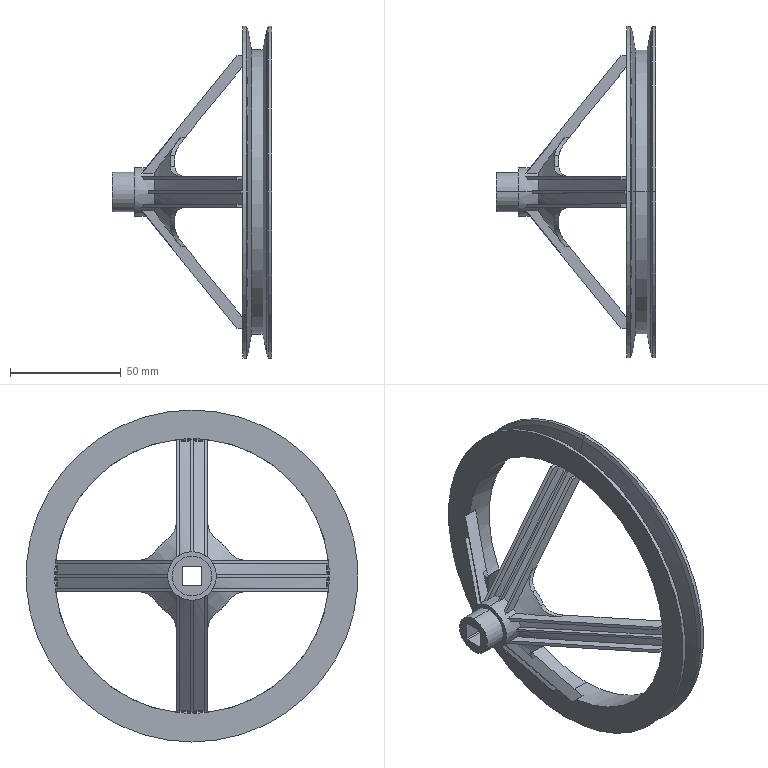Part | SolidWorks | features ICE 6, CirPattern 2, Fillet 1, MirrorPattern 1, Revolution 1 | 1 solid | 195 faces | box 72 x 150 x 150 mm | volume 52845 mm3 | plane 121 | cylinder 36 | cone 22 | torus 16 | commonest cylinder face diameters 124 x10 20 x8 12 x4 40 x4 150 x4 18 x2